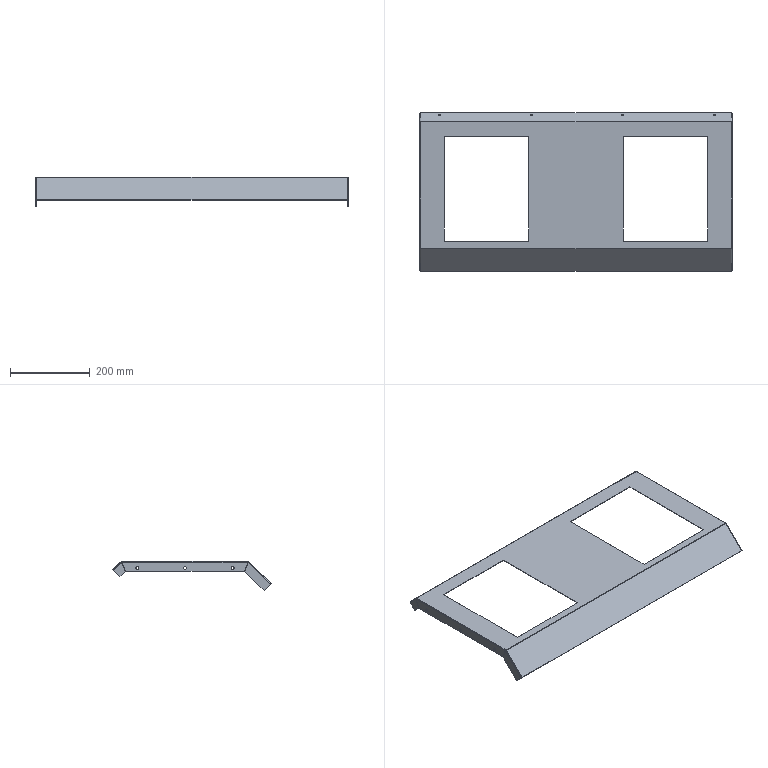Part | SolidWorks | features EdgeFlange 3, HoleWzd 2, FlatPattern 1, ICE 1, SMBaseFlange 1, SheetMetal 1 | 1 solid | 98 faces | box 785 x 397.782 x 74.246 mm | volume 291656 mm3 | plane 54 | cylinder 36 | spline 8 | commonest cylinder face diameters 7 x12 2 x8 4.4 x8 5 x8